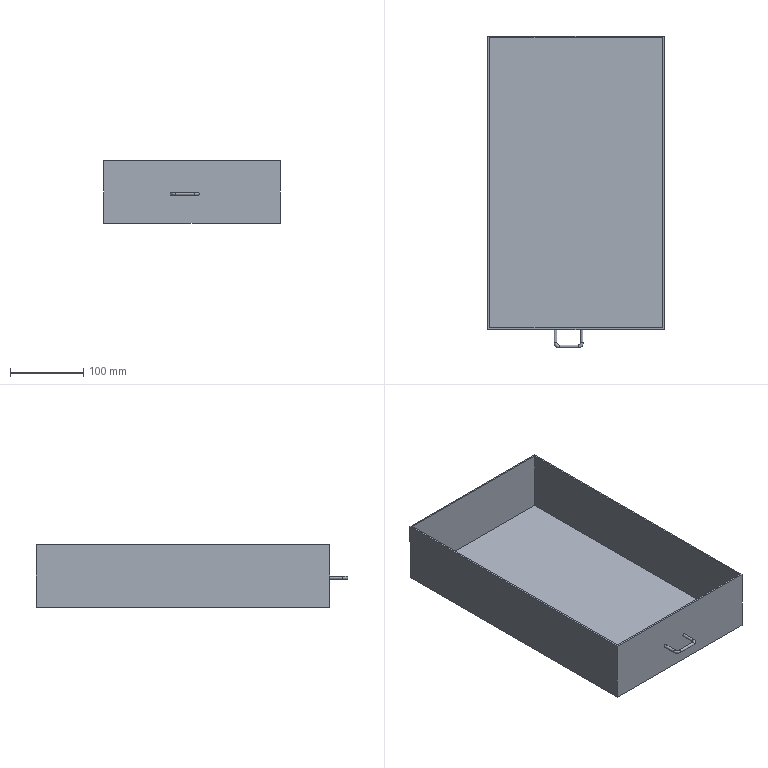Part | NX | features solid 2 | 1 solid | 16 faces | box 240 x 425 x 85 mm | volume 476906 mm3 | plane 11 | cylinder 3 | torus 2 | commonest cylinder face diameters 4 x3
STEP:
#1=CARTESIAN_POINT('',(-448.,-305.,-242.));
#2=VERTEX_POINT('',#1);
#3=CARTESIAN_POINT('',(-448.,-305.,-240.));
#4=DIRECTION('',(0.,-1.,0.));
#5=DIRECTION('',(0.,0.,-1.));
#6=AXIS2_PLACEMENT_3D('',#3,#4,#5);
#7=CIRCLE('',#6,2.);
#8=EDGE_CURVE('',#2,#2,#7,.F.);
#9=ORIENTED_EDGE('',*,*,#8,.T.);
#10=EDGE_LOOP('',(#9));
#11=FACE_BOUND('',#10,.T.);
#12=CARTESIAN_POINT('',(-540.,-305.,-195.));
#13=VERTEX_POINT('',#12);
#14=CARTESIAN_POINT('',(-300.,-305.,-195.));
#15=VERTEX_POINT('',#14);
#16=CARTESIAN_POINT('',(-540.,-305.,-195.));
#17=DIRECTION('',(1.,0.,0.));
#18=VECTOR('',#17,1000.);
#19=LINE('',#16,#18);
#20=EDGE_CURVE('',#13,#15,#19,.T.);
#21=ORIENTED_EDGE('',*,*,#20,.F.);
#22=CARTESIAN_POINT('',(-540.,-305.,-280.));
#23=VERTEX_POINT('',#22);
#24=CARTESIAN_POINT('',(-540.,-305.,-215.));
#25=DIRECTION('',(0.,0.,-1.));
#26=VECTOR('',#25,1000.);
#27=LINE('',#24,#26);
#28=EDGE_CURVE('',#13,#23,#27,.T.);
#29=ORIENTED_EDGE('',*,*,#28,.T.);
#30=CARTESIAN_POINT('',(-300.,-305.,-280.));
#31=VERTEX_POINT('',#30);
#32=CARTESIAN_POINT('',(-540.,-305.,-280.));
#33=DIRECTION('',(1.,0.,0.));
#34=VECTOR('',#33,1000.);
#35=LINE('',#32,#34);
#36=EDGE_CURVE('',#23,#31,#35,.T.);
#37=ORIENTED_EDGE('',*,*,#36,.T.);
#38=CARTESIAN_POINT('',(-300.,-305.,-215.));
#39=DIRECTION('',(0.,0.,1.));
#40=VECTOR('',#39,1000.);
#41=LINE('',#38,#40);
#42=EDGE_CURVE('',#15,#31,#41,.F.);
#43=ORIENTED_EDGE('',*,*,#42,.F.);
#44=EDGE_LOOP('',(#21,#29,#37,#43));
#45=FACE_BOUND('',#44,.T.);
#46=CARTESIAN_POINT('',(-412.,-305.,-238.));
#47=VERTEX_POINT('',#46);
#48=CARTESIAN_POINT('',(-412.,-305.,-240.));
#49=DIRECTION('',(0.,1.,0.));
#50=DIRECTION('',(0.,0.,1.));
#51=AXIS2_PLACEMENT_3D('',#48,#49,#50);
#52=CIRCLE('',#51,2.);
#53=EDGE_CURVE('',#47,#47,#52,.F.);
#54=ORIENTED_EDGE('',*,*,#53,.F.);
#55=EDGE_LOOP('',(#54));
#56=FACE_BOUND('',#55,.T.);
#57=CARTESIAN_POINT('',(-540.,-305.,-215.));
#58=DIRECTION('',(0.,1.,0.));
#59=DIRECTION('',(0.,0.,1.));
#60=AXIS2_PLACEMENT_3D('',#57,#58,#59);
#61=PLANE('',#60);
#62=ADVANCED_FACE('',(#11,#45,#56),#61,.F.);
#63=CARTESIAN_POINT('',(-300.,95.,-195.));
#64=VERTEX_POINT('',#63);
#65=CARTESIAN_POINT('',(-300.,0.,-195.));
#66=DIRECTION('',(0.,-1.,0.));
#67=VECTOR('',#66,1000.);
#68=LINE('',#65,#67);
#69=EDGE_CURVE('',#15,#64,#68,.F.);
#70=ORIENTED_EDGE('',*,*,#69,.F.);
#71=ORIENTED_EDGE('',*,*,#42,.T.);
#72=CARTESIAN_POINT('',(-300.,95.,-280.));
#73=VERTEX_POINT('',#72);
#74=CARTESIAN_POINT('',(-300.,47.5,-280.));
#75=DIRECTION('',(0.,-1.,0.));
#76=VECTOR('',#75,1000.);
#77=LINE('',#74,#76);
#78=EDGE_CURVE('',#31,#73,#77,.F.);
#79=ORIENTED_EDGE('',*,*,#78,.T.);
#80=CARTESIAN_POINT('',(-300.,95.,-125.));
#81=DIRECTION('',(0.,0.,-1.));
#82=VECTOR('',#81,1000.);
#83=LINE('',#80,#82);
#84=EDGE_CURVE('',#64,#73,#83,.T.);
#85=ORIENTED_EDGE('',*,*,#84,.F.);
#86=EDGE_LOOP('',(#70,#71,#79,#85));
#87=FACE_BOUND('',#86,.T.);
#88=CARTESIAN_POINT('',(-300.,405.,-375.));
#89=DIRECTION('',(-1.,0.,0.));
#90=DIRECTION('',(0.,0.,1.));
#91=AXIS2_PLACEMENT_3D('',#88,#89,#90);
#92=PLANE('',#91);
#93=ADVANCED_FACE('',(#87),#92,.F.);
#94=CARTESIAN_POINT('',(-540.,95.,-195.));
#95=VERTEX_POINT('',#94);
#96=CARTESIAN_POINT('',(-540.,-302.5,-195.));
#97=DIRECTION('',(0.,-1.,0.));
#98=VECTOR('',#97,1000.);
#99=LINE('',#96,#98);
#100=EDGE_CURVE('',#95,#13,#99,.T.);
#101=ORIENTED_EDGE('',*,*,#100,.F.);
#102=CARTESIAN_POINT('',(-540.,95.,-280.));
#103=VERTEX_POINT('',#102);
#104=CARTESIAN_POINT('',(-540.,95.,-125.));
#105=DIRECTION('',(0.,0.,1.));
#106=VECTOR('',#105,1000.);
#107=LINE('',#104,#106);
#108=EDGE_CURVE('',#95,#103,#107,.F.);
#109=ORIENTED_EDGE('',*,*,#108,.T.);
#110=CARTESIAN_POINT('',(-540.,-302.5,-280.));
#111=DIRECTION('',(0.,-1.,0.));
#112=VECTOR('',#111,1000.);
#113=LINE('',#110,#112);
#114=EDGE_CURVE('',#103,#23,#113,.T.);
#115=ORIENTED_EDGE('',*,*,#114,.T.);
#116=ORIENTED_EDGE('',*,*,#28,.F.);
#117=EDGE_LOOP('',(#101,#109,#115,#116));
#118=FACE_BOUND('',#117,.T.);
#119=CARTESIAN_POINT('',(-540.,-302.5,-215.));
#120=DIRECTION('',(1.,0.,0.));
#121=DIRECTION('',(0.,0.,-1.));
#122=AXIS2_PLACEMENT_3D('',#119,#120,#121);
#123=PLANE('',#122);
#124=ADVANCED_FACE('',(#118),#123,.F.);
#125=CARTESIAN_POINT('',(0.,95.,-195.));
#126=DIRECTION('',(1.,0.,0.));
#127=VECTOR('',#126,1000.);
#128=LINE('',#125,#127);
#129=EDGE_CURVE('',#64,#95,#128,.F.);
#130=ORIENTED_EDGE('',*,*,#129,.F.);
#131=ORIENTED_EDGE('',*,*,#84,.T.);
#132=CARTESIAN_POINT('',(-362.5,95.,-280.));
#133=DIRECTION('',(1.,0.,0.));
#134=VECTOR('',#133,1000.);
#135=LINE('',#132,#134);
#136=EDGE_CURVE('',#73,#103,#135,.F.);
#137=ORIENTED_EDGE('',*,*,#136,.T.);
#138=ORIENTED_EDGE('',*,*,#108,.F.);
#139=EDGE_LOOP('',(#130,#131,#137,#138));
#140=FACE_BOUND('',#139,.T.);
#141=CARTESIAN_POINT('',(-640.,95.,-125.));
#142=DIRECTION('',(0.,-1.,0.));
#143=DIRECTION('',(1.,0.,0.));
#144=AXIS2_PLACEMENT_3D('',#141,#142,#143);
#145=PLANE('',#144);
#146=ADVANCED_FACE('',(#140),#145,.F.);
#147=ORIENTED_EDGE('',*,*,#136,.F.);
#148=ORIENTED_EDGE('',*,*,#78,.F.);
#149=ORIENTED_EDGE('',*,*,#36,.F.);
#150=ORIENTED_EDGE('',*,*,#114,.F.);
#151=EDGE_LOOP('',(#147,#148,#149,#150));
#152=FACE_BOUND('',#151,.T.);
#153=CARTESIAN_POINT('',(-362.5,47.5,-280.));
#154=DIRECTION('',(0.,0.,1.));
#155=DIRECTION('',(1.,0.,0.));
#156=AXIS2_PLACEMENT_3D('',#153,#154,#155);
#157=PLANE('',#156);
#158=ADVANCED_FACE('',(#152),#157,.F.);
#159=CARTESIAN_POINT('',(-302.,-302.5,-195.));
#160=VERTEX_POINT('',#159);
#161=CARTESIAN_POINT('',(-537.5,-302.5,-195.));
#162=VERTEX_POINT('',#161);
#163=CARTESIAN_POINT('',(-360.,-302.5,-195.));
#164=DIRECTION('',(-1.,0.,0.));
#165=VECTOR('',#164,1000.);
#166=LINE('',#163,#165);
#167=EDGE_CURVE('',#160,#162,#166,.T.);
#168=ORIENTED_EDGE('',*,*,#167,.T.);
#169=CARTESIAN_POINT('',(-537.5,93.,-195.));
#170=VERTEX_POINT('',#169);
#171=CARTESIAN_POINT('',(-537.5,-302.5,-195.));
#172=DIRECTION('',(0.,1.,0.));
#173=VECTOR('',#172,1000.);
#174=LINE('',#171,#173);
#175=EDGE_CURVE('',#162,#170,#174,.T.);
#176=ORIENTED_EDGE('',*,*,#175,.T.);
#177=CARTESIAN_POINT('',(-302.,93.,-195.));
#178=VERTEX_POINT('',#177);
#179=CARTESIAN_POINT('',(-540.,93.,-195.));
#180=DIRECTION('',(1.,0.,0.));
#181=VECTOR('',#180,1000.);
#182=LINE('',#179,#181);
#183=EDGE_CURVE('',#170,#178,#182,.T.);
#184=ORIENTED_EDGE('',*,*,#183,.T.);
#185=CARTESIAN_POINT('',(-302.,47.5,-195.));
#186=DIRECTION('',(0.,-1.,0.));
#187=VECTOR('',#186,1000.);
#188=LINE('',#185,#187);
#189=EDGE_CURVE('',#178,#160,#188,.T.);
#190=ORIENTED_EDGE('',*,*,#189,.T.);
#191=EDGE_LOOP('',(#168,#176,#184,#190));
#192=FACE_BOUND('',#191,.T.);
#193=ORIENTED_EDGE('',*,*,#100,.T.);
#194=ORIENTED_EDGE('',*,*,#20,.T.);
#195=ORIENTED_EDGE('',*,*,#69,.T.);
#196=ORIENTED_EDGE('',*,*,#129,.T.);
#197=EDGE_LOOP('',(#193,#194,#195,#196));
#198=FACE_BOUND('',#197,.T.);
#199=CARTESIAN_POINT('',(0.,0.,-195.));
#200=DIRECTION('',(0.,0.,1.));
#201=DIRECTION('',(1.,0.,0.));
#202=AXIS2_PLACEMENT_3D('',#199,#200,#201);
#203=PLANE('',#202);
#204=ADVANCED_FACE('',(#192,#198),#203,.T.);
#205=CARTESIAN_POINT('',(-302.,-302.5,-277.5));
#206=VERTEX_POINT('',#205);
#207=CARTESIAN_POINT('',(-302.,93.,-277.5));
#208=VERTEX_POINT('',#207);
#209=CARTESIAN_POINT('',(-302.,-302.5,-277.5));
#210=DIRECTION('',(0.,1.,0.));
#211=VECTOR('',#210,1000.);
#212=LINE('',#209,#211);
#213=EDGE_CURVE('',#206,#208,#212,.T.);
#214=ORIENTED_EDGE('',*,*,#213,.T.);
#215=CARTESIAN_POINT('',(-537.5,93.,-277.5));
#216=VERTEX_POINT('',#215);
#217=CARTESIAN_POINT('',(-362.5,93.,-277.5));
#218=DIRECTION('',(-1.,0.,0.));
#219=VECTOR('',#218,1000.);
#220=LINE('',#217,#219);
#221=EDGE_CURVE('',#208,#216,#220,.T.);
#222=ORIENTED_EDGE('',*,*,#221,.T.);
#223=CARTESIAN_POINT('',(-537.5,-302.5,-277.5));
#224=VERTEX_POINT('',#223);
#225=CARTESIAN_POINT('',(-537.5,47.5,-277.5));
#226=DIRECTION('',(0.,-1.,0.));
#227=VECTOR('',#226,1000.);
#228=LINE('',#225,#227);
#229=EDGE_CURVE('',#216,#224,#228,.T.);
#230=ORIENTED_EDGE('',*,*,#229,.T.);
#231=CARTESIAN_POINT('',(-537.5,-302.5,-277.5));
#232=DIRECTION('',(1.,0.,0.));
#233=VECTOR('',#232,1000.);
#234=LINE('',#231,#233);
#235=EDGE_CURVE('',#224,#206,#234,.T.);
#236=ORIENTED_EDGE('',*,*,#235,.T.);
#237=EDGE_LOOP('',(#214,#222,#230,#236));
#238=FACE_BOUND('',#237,.T.);
#239=CARTESIAN_POINT('',(-362.5,47.5,-277.5));
#240=DIRECTION('',(0.,0.,1.));
#241=DIRECTION('',(1.,0.,0.));
#242=AXIS2_PLACEMENT_3D('',#239,#240,#241);
#243=PLANE('',#242);
#244=ADVANCED_FACE('',(#238),#243,.T.);
#245=ORIENTED_EDGE('',*,*,#189,.F.);
#246=CARTESIAN_POINT('',(-302.,93.,-215.));
#247=DIRECTION('',(0.,0.,-1.));
#248=VECTOR('',#247,1000.);
#249=LINE('',#246,#248);
#250=EDGE_CURVE('',#178,#208,#249,.T.);
#251=ORIENTED_EDGE('',*,*,#250,.T.);
#252=ORIENTED_EDGE('',*,*,#213,.F.);
#253=CARTESIAN_POINT('',(-302.,-302.5,-215.));
#254=DIRECTION('',(0.,0.,-1.));
#255=VECTOR('',#254,1000.);
#256=LINE('',#253,#255);
#257=EDGE_CURVE('',#160,#206,#256,.T.);
#258=ORIENTED_EDGE('',*,*,#257,.F.);
#259=EDGE_LOOP('',(#245,#251,#252,#258));
#260=FACE_BOUND('',#259,.T.);
#261=CARTESIAN_POINT('',(-302.,47.5,-215.));
#262=DIRECTION('',(1.,0.,0.));
#263=DIRECTION('',(0.,0.,-1.));
#264=AXIS2_PLACEMENT_3D('',#261,#262,#263);
#265=PLANE('',#264);
#266=ADVANCED_FACE('',(#260),#265,.F.);
#267=ORIENTED_EDGE('',*,*,#175,.F.);
#268=CARTESIAN_POINT('',(-537.5,-302.5,-215.));
#269=DIRECTION('',(0.,0.,-1.));
#270=VECTOR('',#269,1000.);
#271=LINE('',#268,#270);
#272=EDGE_CURVE('',#162,#224,#271,.T.);
#273=ORIENTED_EDGE('',*,*,#272,.T.);
#274=ORIENTED_EDGE('',*,*,#229,.F.);
#275=CARTESIAN_POINT('',(-537.5,93.,-215.));
#276=DIRECTION('',(0.,0.,-1.));
#277=VECTOR('',#276,1000.);
#278=LINE('',#275,#277);
#279=EDGE_CURVE('',#170,#216,#278,.T.);
#280=ORIENTED_EDGE('',*,*,#279,.F.);
#281=EDGE_LOOP('',(#267,#273,#274,#280));
#282=FACE_BOUND('',#281,.T.);
#283=CARTESIAN_POINT('',(-537.5,-302.5,-215.));
#284=DIRECTION('',(-1.,0.,0.));
#285=DIRECTION('',(0.,0.,1.));
#286=AXIS2_PLACEMENT_3D('',#283,#284,#285);
#287=PLANE('',#286);
#288=ADVANCED_FACE('',(#282),#287,.F.);
#289=ORIENTED_EDGE('',*,*,#183,.F.);
#290=ORIENTED_EDGE('',*,*,#279,.T.);
#291=ORIENTED_EDGE('',*,*,#221,.F.);
#292=ORIENTED_EDGE('',*,*,#250,.F.);
#293=EDGE_LOOP('',(#289,#290,#291,#292));
#294=FACE_BOUND('',#293,.T.);
#295=CARTESIAN_POINT('',(-540.,93.,-215.));
#296=DIRECTION('',(0.,1.,0.));
#297=DIRECTION('',(0.,0.,1.));
#298=AXIS2_PLACEMENT_3D('',#295,#296,#297);
#299=PLANE('',#298);
#300=ADVANCED_FACE('',(#294),#299,.F.);
#301=ORIENTED_EDGE('',*,*,#167,.F.);
#302=ORIENTED_EDGE('',*,*,#257,.T.);
#303=ORIENTED_EDGE('',*,*,#235,.F.);
#304=ORIENTED_EDGE('',*,*,#272,.F.);
#305=EDGE_LOOP('',(#301,#302,#303,#304));
#306=FACE_BOUND('',#305,.T.);
#307=CARTESIAN_POINT('',(-360.,-302.5,-215.));
#308=DIRECTION('',(0.,-1.,0.));
#309=DIRECTION('',(0.,0.,-1.));
#310=AXIS2_PLACEMENT_3D('',#307,#308,#309);
#311=PLANE('',#310);
#312=ADVANCED_FACE('',(#306),#311,.F.);
#313=CARTESIAN_POINT('',(-443.,-328.,-242.));
#314=VERTEX_POINT('',#313);
#315=CARTESIAN_POINT('',(-443.,-328.,-240.));
#316=DIRECTION('',(-1.,0.,0.));
#317=DIRECTION('',(0.,0.,-1.));
#318=AXIS2_PLACEMENT_3D('',#315,#316,#317);
#319=CIRCLE('',#318,2.);
#320=EDGE_CURVE('',#314,#314,#319,.T.);
#321=ORIENTED_EDGE('',*,*,#320,.T.);
#322=EDGE_LOOP('',(#321));
#323=FACE_BOUND('',#322,.T.);
#324=CARTESIAN_POINT('',(-448.,-323.,-242.));
#325=VERTEX_POINT('',#324);
#326=CARTESIAN_POINT('',(-448.,-323.,-240.));
#327=DIRECTION('',(0.,1.,0.));
#328=DIRECTION('',(0.,0.,-1.));
#329=AXIS2_PLACEMENT_3D('',#326,#327,#328);
#330=CIRCLE('',#329,2.);
#331=EDGE_CURVE('',#325,#325,#330,.T.);
#332=ORIENTED_EDGE('',*,*,#331,.F.);
#333=EDGE_LOOP('',(#332));
#334=FACE_BOUND('',#333,.T.);
#335=CARTESIAN_POINT('',(-443.,-323.,-240.));
#336=DIRECTION('',(0.,0.,-1.));
#337=DIRECTION('',(-1.,0.,0.));
#338=AXIS2_PLACEMENT_3D('',#335,#336,#337);
#339=TOROIDAL_SURFACE('',#338,5.,2.);
#340=ADVANCED_FACE('',(#323,#334),#339,.T.);
#341=ORIENTED_EDGE('',*,*,#331,.T.);
#342=EDGE_LOOP('',(#341));
#343=FACE_BOUND('',#342,.T.);
#344=ORIENTED_EDGE('',*,*,#8,.F.);
#345=EDGE_LOOP('',(#344));
#346=FACE_BOUND('',#345,.T.);
#347=CARTESIAN_POINT('',(-448.,-323.,-240.));
#348=DIRECTION('',(0.,1.,0.));
#349=DIRECTION('',(0.,0.,1.));
#350=AXIS2_PLACEMENT_3D('',#347,#348,#349);
#351=CYLINDRICAL_SURFACE('',#350,2.);
#352=ADVANCED_FACE('',(#343,#346),#351,.T.);
#353=CARTESIAN_POINT('',(-417.,-328.,-242.));
#354=VERTEX_POINT('',#353);
#355=CARTESIAN_POINT('',(-417.,-328.,-240.));
#356=DIRECTION('',(-1.,0.,0.));
#357=DIRECTION('',(0.,0.,-1.));
#358=AXIS2_PLACEMENT_3D('',#355,#356,#357);
#359=CIRCLE('',#358,2.);
#360=EDGE_CURVE('',#354,#354,#359,.T.);
#361=ORIENTED_EDGE('',*,*,#360,.T.);
#362=EDGE_LOOP('',(#361));
#363=FACE_BOUND('',#362,.T.);
#364=ORIENTED_EDGE('',*,*,#320,.F.);
#365=EDGE_LOOP('',(#364));
#366=FACE_BOUND('',#365,.T.);
#367=CARTESIAN_POINT('',(-417.,-328.,-240.));
#368=DIRECTION('',(-1.,0.,0.));
#369=DIRECTION('',(0.,0.,1.));
#370=AXIS2_PLACEMENT_3D('',#367,#368,#369);
#371=CYLINDRICAL_SURFACE('',#370,2.);
#372=ADVANCED_FACE('',(#363,#366),#371,.T.);
#373=CARTESIAN_POINT('',(-412.,-323.,-242.));
#374=VERTEX_POINT('',#373);
#375=CARTESIAN_POINT('',(-412.,-323.,-240.));
#376=DIRECTION('',(0.,-1.,0.));
#377=DIRECTION('',(0.,0.,-1.));
#378=AXIS2_PLACEMENT_3D('',#375,#376,#377);
#379=CIRCLE('',#378,2.);
#380=EDGE_CURVE('',#374,#374,#379,.T.);
#381=ORIENTED_EDGE('',*,*,#380,.T.);
#382=EDGE_LOOP('',(#381));
#383=FACE_BOUND('',#382,.T.);
#384=ORIENTED_EDGE('',*,*,#360,.F.);
#385=EDGE_LOOP('',(#384));
#386=FACE_BOUND('',#385,.T.);
#387=CARTESIAN_POINT('',(-417.,-323.,-240.));
#388=DIRECTION('',(0.,0.,-1.));
#389=DIRECTION('',(-1.,0.,0.));
#390=AXIS2_PLACEMENT_3D('',#387,#388,#389);
#391=TOROIDAL_SURFACE('',#390,5.,2.);
#392=ADVANCED_FACE('',(#383,#386),#391,.T.);
#393=ORIENTED_EDGE('',*,*,#380,.F.);
#394=EDGE_LOOP('',(#393));
#395=FACE_BOUND('',#394,.T.);
#396=ORIENTED_EDGE('',*,*,#53,.T.);
#397=EDGE_LOOP('',(#396));
#398=FACE_BOUND('',#397,.T.);
#399=CARTESIAN_POINT('',(-412.,-323.,-240.));
#400=DIRECTION('',(0.,1.,0.));
#401=DIRECTION('',(0.,0.,1.));
#402=AXIS2_PLACEMENT_3D('',#399,#400,#401);
#403=CYLINDRICAL_SURFACE('',#402,2.);
#404=ADVANCED_FACE('',(#395,#398),#403,.T.);
#405=CLOSED_SHELL('',(#62,#93,#124,#146,#158,#204,#244,#266,#288,#300,#312,#340,#352,#372,#392,#404));
#406=MANIFOLD_SOLID_BREP('',#405);
#407=(LENGTH_UNIT()NAMED_UNIT(*)SI_UNIT(.MILLI.,.METRE.));
#408=UNCERTAINTY_MEASURE_WITH_UNIT(LENGTH_MEASURE(0.00001),#407,'','');
#409=(NAMED_UNIT(*)PLANE_ANGLE_UNIT()SI_UNIT($,.RADIAN.));
#410=(NAMED_UNIT(*)SI_UNIT($,.STERADIAN.)SOLID_ANGLE_UNIT());
#411=(GEOMETRIC_REPRESENTATION_CONTEXT(3)GLOBAL_UNCERTAINTY_ASSIGNED_CONTEXT((#408))GLOBAL_UNIT_ASSIGNED_CONTEXT((#407,#409,#410))REPRESENTATION_CONTEXT('',''));
#412=ADVANCED_BREP_SHAPE_REPRESENTATION('',(#406),#411);